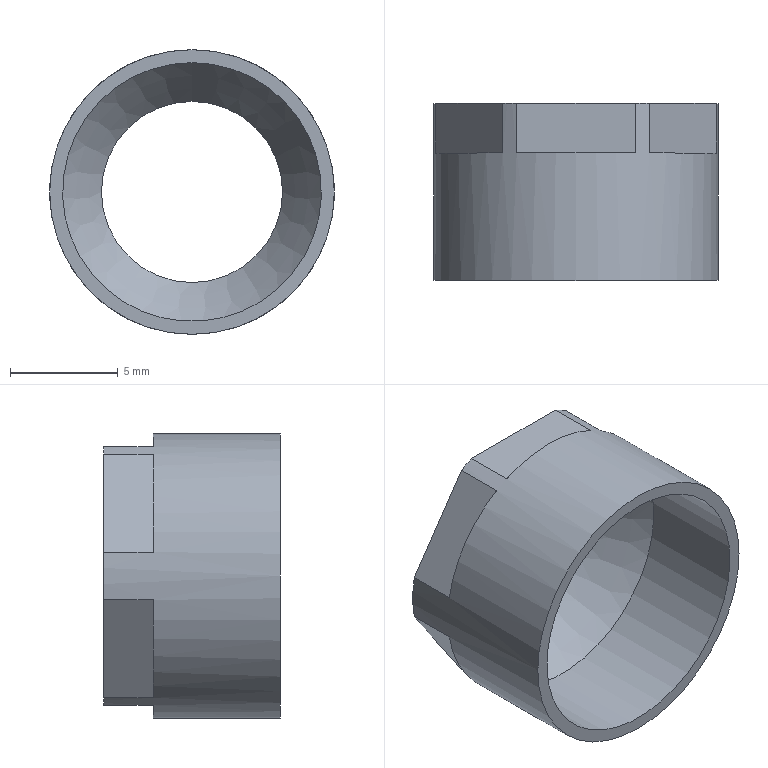Part | STEP file | 1 solid | 18 faces | box 13.2 x 8.2 x 13.2 mm | volume 283.542 mm3 | plane 14 | cylinder 3 | cone 1 | commonest cylinder face diameters 8.4 x1 12 x1 13.2 x1
STEP:
#1=CARTESIAN_POINT('',(0.,0.,0.));
#2=DIRECTION('',(0.,0.,1.));
#3=DIRECTION('',(1.,0.,0.));
#4=AXIS2_PLACEMENT_3D('',#1,#2,#3);
#5=CARTESIAN_POINT('',(0.,0.,6.6));
#6=VERTEX_POINT('',#5);
#7=CARTESIAN_POINT('',(0.,0.,0.));
#8=DIRECTION('',(0.,1.,0.));
#9=DIRECTION('',(0.,0.,1.));
#10=AXIS2_PLACEMENT_3D('',#7,#8,#9);
#11=CIRCLE('',#10,6.6);
#12=CARTESIAN_POINT('',(0.,-0.41,0.));
#13=DIRECTION('',(0.,1.,0.));
#14=DIRECTION('',(0.,0.,1.));
#15=AXIS2_PLACEMENT_3D('',#12,#13,#14);
#16=CYLINDRICAL_SURFACE('',#15,6.6);
#17=CARTESIAN_POINT('',(0.,0.41));
#18=DIRECTION('',(1.,0.));
#19=VECTOR('',#18,1.);
#20=LINE('',#17,#19);
#21=(GEOMETRIC_REPRESENTATION_CONTEXT(2)PARAMETRIC_REPRESENTATION_CONTEXT()REPRESENTATION_CONTEXT('',''));
#22=DEFINITIONAL_REPRESENTATION('',(#20),#21);
#23=PCURVE('',#16,#22);
#24=CARTESIAN_POINT('',(0.,0.,0.));
#25=DIRECTION('',(0.,1.,0.));
#26=DIRECTION('',(0.,0.,1.));
#27=AXIS2_PLACEMENT_3D('',#24,#25,#26);
#28=PLANE('',#27);
#29=CARTESIAN_POINT('',(0.,0.));
#30=DIRECTION('',(1.,0.));
#31=AXIS2_PLACEMENT_2D('',#29,#30);
#32=CIRCLE('',#31,6.6);
#33=(GEOMETRIC_REPRESENTATION_CONTEXT(2)PARAMETRIC_REPRESENTATION_CONTEXT()REPRESENTATION_CONTEXT('',''));
#34=DEFINITIONAL_REPRESENTATION('',(#32),#33);
#35=PCURVE('',#28,#34);
#36=SURFACE_CURVE('',#11,(#23,#35),.PCURVE_S1.);
#37=EDGE_CURVE('',#6,#6,#36,.T.);
#38=ORIENTED_EDGE('',*,*,#37,.T.);
#39=CARTESIAN_POINT('',(0.,5.9,6.6));
#40=VERTEX_POINT('',#39);
#41=CARTESIAN_POINT('',(0.,0.,6.6));
#42=CARTESIAN_POINT('',(0.,5.9,6.6));
#43=B_SPLINE_CURVE_WITH_KNOTS('',1,(#41,#42),.UNSPECIFIED.,.F.,.F.,(2,2),(0.41,6.31),.PIECEWISE_BEZIER_KNOTS.);
#44=CARTESIAN_POINT('',(6.283,0.));
#45=DIRECTION('',(0.,1.));
#46=VECTOR('',#45,1.);
#47=LINE('',#44,#46);
#48=(GEOMETRIC_REPRESENTATION_CONTEXT(2)PARAMETRIC_REPRESENTATION_CONTEXT()REPRESENTATION_CONTEXT('',''));
#49=DEFINITIONAL_REPRESENTATION('',(#47),#48);
#50=PCURVE('',#16,#49);
#51=CARTESIAN_POINT('',(0.,0.));
#52=DIRECTION('',(0.,1.));
#53=VECTOR('',#52,1.);
#54=LINE('',#51,#53);
#55=(GEOMETRIC_REPRESENTATION_CONTEXT(2)PARAMETRIC_REPRESENTATION_CONTEXT()REPRESENTATION_CONTEXT('',''));
#56=DEFINITIONAL_REPRESENTATION('',(#54),#55);
#57=PCURVE('',#16,#56);
#58=SEAM_CURVE('',#43,(#50,#57),.PCURVE_S1.);
#59=EDGE_CURVE('',#6,#40,#58,.T.);
#60=ORIENTED_EDGE('',*,*,#59,.T.);
#61=CARTESIAN_POINT('',(-2.75,5.9,6.));
#62=VERTEX_POINT('',#61);
#63=CARTESIAN_POINT('',(0.,5.9,0.));
#64=DIRECTION('',(0.,-1.,0.));
#65=DIRECTION('',(0.,0.,1.));
#66=AXIS2_PLACEMENT_3D('',#63,#64,#65);
#67=CIRCLE('',#66,6.6);
#68=CARTESIAN_POINT('',(12.566,6.31));
#69=DIRECTION('',(-1.,0.));
#70=VECTOR('',#69,1.);
#71=LINE('',#68,#70);
#72=(GEOMETRIC_REPRESENTATION_CONTEXT(2)PARAMETRIC_REPRESENTATION_CONTEXT()REPRESENTATION_CONTEXT('',''));
#73=DEFINITIONAL_REPRESENTATION('',(#71),#72);
#74=PCURVE('',#16,#73);
#75=CARTESIAN_POINT('',(0.,5.9,0.));
#76=DIRECTION('',(0.,1.,0.));
#77=DIRECTION('',(0.,0.,1.));
#78=AXIS2_PLACEMENT_3D('',#75,#76,#77);
#79=PLANE('',#78);
#80=CARTESIAN_POINT('',(6.6,0.));
#81=CARTESIAN_POINT('',(6.6,-11.432));
#82=CARTESIAN_POINT('',(-3.3,-5.716));
#83=CARTESIAN_POINT('',(-13.2,0.));
#84=CARTESIAN_POINT('',(-3.3,5.716));
#85=CARTESIAN_POINT('',(6.6,11.432));
#86=CARTESIAN_POINT('',(6.6,0.));
#87=(BOUNDED_CURVE()B_SPLINE_CURVE(2,(#80,#81,#82,#83,#84,#85,#86),.UNSPECIFIED.,.T.,.F.)B_SPLINE_CURVE_WITH_KNOTS((1,2,2,2,2,1),(-2.094,0.,2.094,4.189,6.283,8.378),.UNSPECIFIED.)CURVE()GEOMETRIC_REPRESENTATION_ITEM()RATIONAL_B_SPLINE_CURVE((1.,0.5,1.,0.5,1.,0.5,1.))REPRESENTATION_ITEM(''));
#88=(GEOMETRIC_REPRESENTATION_CONTEXT(2)PARAMETRIC_REPRESENTATION_CONTEXT()REPRESENTATION_CONTEXT('',''));
#89=DEFINITIONAL_REPRESENTATION('',(#87),#88);
#90=PCURVE('',#79,#89);
#91=SURFACE_CURVE('',#67,(#74,#90),.PCURVE_S1.);
#92=EDGE_CURVE('',#40,#62,#91,.T.);
#93=ORIENTED_EDGE('',*,*,#92,.T.);
#94=CARTESIAN_POINT('',(-2.75,8.2,6.));
#95=VERTEX_POINT('',#94);
#96=CARTESIAN_POINT('',(-2.75,-0.41,6.));
#97=DIRECTION('',(0.,1.,0.));
#98=VECTOR('',#97,1.);
#99=LINE('',#96,#98);
#100=CARTESIAN_POINT('',(5.853,0.));
#101=DIRECTION('',(0.,1.));
#102=VECTOR('',#101,1.);
#103=LINE('',#100,#102);
#104=(GEOMETRIC_REPRESENTATION_CONTEXT(2)PARAMETRIC_REPRESENTATION_CONTEXT()REPRESENTATION_CONTEXT('',''));
#105=DEFINITIONAL_REPRESENTATION('',(#103),#104);
#106=PCURVE('',#16,#105);
#107=CARTESIAN_POINT('',(3.169,8.2,6.));
#108=DIRECTION('',(0.,0.,-1.));
#109=DIRECTION('',(-1.,0.,0.));
#110=AXIS2_PLACEMENT_3D('',#107,#108,#109);
#111=PLANE('',#110);
#112=CARTESIAN_POINT('',(5.919,-8.61));
#113=DIRECTION('',(0.,1.));
#114=VECTOR('',#113,1.);
#115=LINE('',#112,#114);
#116=(GEOMETRIC_REPRESENTATION_CONTEXT(2)PARAMETRIC_REPRESENTATION_CONTEXT()REPRESENTATION_CONTEXT('',''));
#117=DEFINITIONAL_REPRESENTATION('',(#115),#116);
#118=PCURVE('',#111,#117);
#119=SURFACE_CURVE('',#99,(#106,#118),.PCURVE_S1.);
#120=EDGE_CURVE('',#62,#95,#119,.T.);
#121=ORIENTED_EDGE('',*,*,#120,.T.);
#122=CARTESIAN_POINT('',(-3.406,8.2,5.653));
#123=VERTEX_POINT('',#122);
#124=CARTESIAN_POINT('',(0.,8.2,0.));
#125=DIRECTION('',(0.,-1.,0.));
#126=DIRECTION('',(0.,0.,1.));
#127=AXIS2_PLACEMENT_3D('',#124,#125,#126);
#128=CIRCLE('',#127,6.6);
#129=CARTESIAN_POINT('',(6.283,8.61));
#130=DIRECTION('',(-1.,0.));
#131=VECTOR('',#130,1.);
#132=LINE('',#129,#131);
#133=(GEOMETRIC_REPRESENTATION_CONTEXT(2)PARAMETRIC_REPRESENTATION_CONTEXT()REPRESENTATION_CONTEXT('',''));
#134=DEFINITIONAL_REPRESENTATION('',(#132),#133);
#135=PCURVE('',#16,#134);
#136=CARTESIAN_POINT('',(0.,8.2,0.));
#137=DIRECTION('',(0.,1.,0.));
#138=DIRECTION('',(0.,0.,1.));
#139=AXIS2_PLACEMENT_3D('',#136,#137,#138);
#140=PLANE('',#139);
#141=CARTESIAN_POINT('',(6.6,0.));
#142=CARTESIAN_POINT('',(6.6,-11.432));
#143=CARTESIAN_POINT('',(-3.3,-5.716));
#144=CARTESIAN_POINT('',(-13.2,0.));
#145=CARTESIAN_POINT('',(-3.3,5.716));
#146=CARTESIAN_POINT('',(6.6,11.432));
#147=CARTESIAN_POINT('',(6.6,0.));
#148=(BOUNDED_CURVE()B_SPLINE_CURVE(2,(#141,#142,#143,#144,#145,#146,#147),.UNSPECIFIED.,.T.,.F.)B_SPLINE_CURVE_WITH_KNOTS((1,2,2,2,2,1),(-2.094,0.,2.094,4.189,6.283,8.378),.UNSPECIFIED.)CURVE()GEOMETRIC_REPRESENTATION_ITEM()RATIONAL_B_SPLINE_CURVE((1.,0.5,1.,0.5,1.,0.5,1.))REPRESENTATION_ITEM(''));
#149=(GEOMETRIC_REPRESENTATION_CONTEXT(2)PARAMETRIC_REPRESENTATION_CONTEXT()REPRESENTATION_CONTEXT('',''));
#150=DEFINITIONAL_REPRESENTATION('',(#148),#149);
#151=PCURVE('',#140,#150);
#152=SURFACE_CURVE('',#128,(#135,#151),.PCURVE_S1.);
#153=EDGE_CURVE('',#95,#123,#152,.T.);
#154=ORIENTED_EDGE('',*,*,#153,.T.);
#155=CARTESIAN_POINT('',(-3.406,5.9,5.653));
#156=VERTEX_POINT('',#155);
#157=CARTESIAN_POINT('',(-3.406,-0.41,5.653));
#158=DIRECTION('',(0.,-1.,0.));
#159=VECTOR('',#158,1.);
#160=LINE('',#157,#159);
#161=CARTESIAN_POINT('',(5.741,0.));
#162=DIRECTION('',(0.,-1.));
#163=VECTOR('',#162,1.);
#164=LINE('',#161,#163);
#165=(GEOMETRIC_REPRESENTATION_CONTEXT(2)PARAMETRIC_REPRESENTATION_CONTEXT()REPRESENTATION_CONTEXT('',''));
#166=DEFINITIONAL_REPRESENTATION('',(#164),#165);
#167=PCURVE('',#16,#166);
#168=CARTESIAN_POINT('',(-3.169,8.2,6.));
#169=DIRECTION('',(0.826,0.,-0.5637));
#170=DIRECTION('',(-0.5637,0.,-0.826));
#171=AXIS2_PLACEMENT_3D('',#168,#169,#170);
#172=PLANE('',#171);
#173=CARTESIAN_POINT('',(0.4196,-8.61));
#174=DIRECTION('',(0.,-1.));
#175=VECTOR('',#174,1.);
#176=LINE('',#173,#175);
#177=(GEOMETRIC_REPRESENTATION_CONTEXT(2)PARAMETRIC_REPRESENTATION_CONTEXT()REPRESENTATION_CONTEXT('',''));
#178=DEFINITIONAL_REPRESENTATION('',(#176),#177);
#179=PCURVE('',#172,#178);
#180=SURFACE_CURVE('',#160,(#167,#179),.PCURVE_S1.);
#181=EDGE_CURVE('',#123,#156,#180,.T.);
#182=ORIENTED_EDGE('',*,*,#181,.T.);
#183=CARTESIAN_POINT('',(-6.506,5.9,1.111));
#184=VERTEX_POINT('',#183);
#185=CARTESIAN_POINT('',(0.,5.9,0.));
#186=DIRECTION('',(0.,-1.,0.));
#187=DIRECTION('',(0.,0.,1.));
#188=AXIS2_PLACEMENT_3D('',#185,#186,#187);
#189=CIRCLE('',#188,6.6);
#190=CARTESIAN_POINT('',(6.283,6.31));
#191=DIRECTION('',(-1.,0.));
#192=VECTOR('',#191,1.);
#193=LINE('',#190,#192);
#194=(GEOMETRIC_REPRESENTATION_CONTEXT(2)PARAMETRIC_REPRESENTATION_CONTEXT()REPRESENTATION_CONTEXT('',''));
#195=DEFINITIONAL_REPRESENTATION('',(#193),#194);
#196=PCURVE('',#16,#195);
#197=CARTESIAN_POINT('',(0.,5.9,0.));
#198=DIRECTION('',(0.,1.,0.));
#199=DIRECTION('',(0.,0.,1.));
#200=AXIS2_PLACEMENT_3D('',#197,#198,#199);
#201=PLANE('',#200);
#202=CARTESIAN_POINT('',(6.6,0.));
#203=CARTESIAN_POINT('',(6.6,-11.432));
#204=CARTESIAN_POINT('',(-3.3,-5.716));
#205=CARTESIAN_POINT('',(-13.2,0.));
#206=CARTESIAN_POINT('',(-3.3,5.716));
#207=CARTESIAN_POINT('',(6.6,11.432));
#208=CARTESIAN_POINT('',(6.6,0.));
#209=(BOUNDED_CURVE()B_SPLINE_CURVE(2,(#202,#203,#204,#205,#206,#207,#208),.UNSPECIFIED.,.T.,.F.)B_SPLINE_CURVE_WITH_KNOTS((1,2,2,2,2,1),(-2.094,0.,2.094,4.189,6.283,8.378),.UNSPECIFIED.)CURVE()GEOMETRIC_REPRESENTATION_ITEM()RATIONAL_B_SPLINE_CURVE((1.,0.5,1.,0.5,1.,0.5,1.))REPRESENTATION_ITEM(''));
#210=(GEOMETRIC_REPRESENTATION_CONTEXT(2)PARAMETRIC_REPRESENTATION_CONTEXT()REPRESENTATION_CONTEXT('',''));
#211=DEFINITIONAL_REPRESENTATION('',(#209),#210);
#212=PCURVE('',#201,#211);
#213=SURFACE_CURVE('',#189,(#196,#212),.PCURVE_S1.);
#214=EDGE_CURVE('',#156,#184,#213,.T.);
#215=ORIENTED_EDGE('',*,*,#214,.T.);
#216=CARTESIAN_POINT('',(-6.506,8.2,1.111));
#217=VERTEX_POINT('',#216);
#218=CARTESIAN_POINT('',(-6.506,-0.41,1.111));
#219=DIRECTION('',(0.,1.,0.));
#220=VECTOR('',#219,1.);
#221=LINE('',#218,#220);
#222=CARTESIAN_POINT('',(4.882,0.));
#223=DIRECTION('',(0.,1.));
#224=VECTOR('',#223,1.);
#225=LINE('',#222,#224);
#226=(GEOMETRIC_REPRESENTATION_CONTEXT(2)PARAMETRIC_REPRESENTATION_CONTEXT()REPRESENTATION_CONTEXT('',''));
#227=DEFINITIONAL_REPRESENTATION('',(#225),#226);
#228=PCURVE('',#16,#227);
#229=CARTESIAN_POINT('',(5.919,-8.61));
#230=DIRECTION('',(0.,1.));
#231=VECTOR('',#230,1.);
#232=LINE('',#229,#231);
#233=(GEOMETRIC_REPRESENTATION_CONTEXT(2)PARAMETRIC_REPRESENTATION_CONTEXT()REPRESENTATION_CONTEXT('',''));
#234=DEFINITIONAL_REPRESENTATION('',(#232),#233);
#235=PCURVE('',#172,#234);
#236=SURFACE_CURVE('',#221,(#228,#235),.PCURVE_S1.);
#237=EDGE_CURVE('',#184,#217,#236,.T.);
#238=ORIENTED_EDGE('',*,*,#237,.T.);
#239=CARTESIAN_POINT('',(-6.506,8.2,-1.111));
#240=VERTEX_POINT('',#239);
#241=CARTESIAN_POINT('',(0.,8.2,0.));
#242=DIRECTION('',(0.,-1.,0.));
#243=DIRECTION('',(0.,0.,1.));
#244=AXIS2_PLACEMENT_3D('',#241,#242,#243);
#245=CIRCLE('',#244,6.6);
#246=CARTESIAN_POINT('',(6.283,8.61));
#247=DIRECTION('',(-1.,0.));
#248=VECTOR('',#247,1.);
#249=LINE('',#246,#248);
#250=(GEOMETRIC_REPRESENTATION_CONTEXT(2)PARAMETRIC_REPRESENTATION_CONTEXT()REPRESENTATION_CONTEXT('',''));
#251=DEFINITIONAL_REPRESENTATION('',(#249),#250);
#252=PCURVE('',#16,#251);
#253=CARTESIAN_POINT('',(6.6,0.));
#254=CARTESIAN_POINT('',(6.6,-11.432));
#255=CARTESIAN_POINT('',(-3.3,-5.716));
#256=CARTESIAN_POINT('',(-13.2,0.));
#257=CARTESIAN_POINT('',(-3.3,5.716));
#258=CARTESIAN_POINT('',(6.6,11.432));
#259=CARTESIAN_POINT('',(6.6,0.));
#260=(BOUNDED_CURVE()B_SPLINE_CURVE(2,(#253,#254,#255,#256,#257,#258,#259),.UNSPECIFIED.,.T.,.F.)B_SPLINE_CURVE_WITH_KNOTS((1,2,2,2,2,1),(-2.094,0.,2.094,4.189,6.283,8.378),.UNSPECIFIED.)CURVE()GEOMETRIC_REPRESENTATION_ITEM()RATIONAL_B_SPLINE_CURVE((1.,0.5,1.,0.5,1.,0.5,1.))REPRESENTATION_ITEM(''));
#261=(GEOMETRIC_REPRESENTATION_CONTEXT(2)PARAMETRIC_REPRESENTATION_CONTEXT()REPRESENTATION_CONTEXT('',''));
#262=DEFINITIONAL_REPRESENTATION('',(#260),#261);
#263=PCURVE('',#140,#262);
#264=SURFACE_CURVE('',#245,(#252,#263),.PCURVE_S1.);
#265=EDGE_CURVE('',#217,#240,#264,.T.);
#266=ORIENTED_EDGE('',*,*,#265,.T.);
#267=CARTESIAN_POINT('',(-6.506,5.9,-1.111));
#268=VERTEX_POINT('',#267);
#269=CARTESIAN_POINT('',(-6.506,-0.41,-1.111));
#270=DIRECTION('',(0.,-1.,0.));
#271=VECTOR('',#270,1.);
#272=LINE('',#269,#271);
#273=CARTESIAN_POINT('',(4.543,0.));
#274=DIRECTION('',(0.,-1.));
#275=VECTOR('',#274,1.);
#276=LINE('',#273,#275);
#277=(GEOMETRIC_REPRESENTATION_CONTEXT(2)PARAMETRIC_REPRESENTATION_CONTEXT()REPRESENTATION_CONTEXT('',''));
#278=DEFINITIONAL_REPRESENTATION('',(#276),#277);
#279=PCURVE('',#16,#278);
#280=CARTESIAN_POINT('',(-7.264,8.2,0.));
#281=DIRECTION('',(0.826,0.,0.5637));
#282=DIRECTION('',(0.5637,0.,-0.826));
#283=AXIS2_PLACEMENT_3D('',#280,#281,#282);
#284=PLANE('',#283);
#285=CARTESIAN_POINT('',(1.346,-8.61));
#286=DIRECTION('',(0.,-1.));
#287=VECTOR('',#286,1.);
#288=LINE('',#285,#287);
#289=(GEOMETRIC_REPRESENTATION_CONTEXT(2)PARAMETRIC_REPRESENTATION_CONTEXT()REPRESENTATION_CONTEXT('',''));
#290=DEFINITIONAL_REPRESENTATION('',(#288),#289);
#291=PCURVE('',#284,#290);
#292=SURFACE_CURVE('',#272,(#279,#291),.PCURVE_S1.);
#293=EDGE_CURVE('',#240,#268,#292,.T.);
#294=ORIENTED_EDGE('',*,*,#293,.T.);
#295=CARTESIAN_POINT('',(-3.406,5.9,-5.653));
#296=VERTEX_POINT('',#295);
#297=CARTESIAN_POINT('',(0.,5.9,0.));
#298=DIRECTION('',(0.,-1.,0.));
#299=DIRECTION('',(0.,0.,1.));
#300=AXIS2_PLACEMENT_3D('',#297,#298,#299);
#301=CIRCLE('',#300,6.6);
#302=CARTESIAN_POINT('',(6.283,6.31));
#303=DIRECTION('',(-1.,0.));
#304=VECTOR('',#303,1.);
#305=LINE('',#302,#304);
#306=(GEOMETRIC_REPRESENTATION_CONTEXT(2)PARAMETRIC_REPRESENTATION_CONTEXT()REPRESENTATION_CONTEXT('',''));
#307=DEFINITIONAL_REPRESENTATION('',(#305),#306);
#308=PCURVE('',#16,#307);
#309=CARTESIAN_POINT('',(0.,5.9,0.));
#310=DIRECTION('',(0.,1.,0.));
#311=DIRECTION('',(0.,0.,1.));
#312=AXIS2_PLACEMENT_3D('',#309,#310,#311);
#313=PLANE('',#312);
#314=CARTESIAN_POINT('',(6.6,0.));
#315=CARTESIAN_POINT('',(6.6,-11.432));
#316=CARTESIAN_POINT('',(-3.3,-5.716));
#317=CARTESIAN_POINT('',(-13.2,0.));
#318=CARTESIAN_POINT('',(-3.3,5.716));
#319=CARTESIAN_POINT('',(6.6,11.432));
#320=CARTESIAN_POINT('',(6.6,0.));
#321=(BOUNDED_CURVE()B_SPLINE_CURVE(2,(#314,#315,#316,#317,#318,#319,#320),.UNSPECIFIED.,.T.,.F.)B_SPLINE_CURVE_WITH_KNOTS((1,2,2,2,2,1),(-2.094,0.,2.094,4.189,6.283,8.378),.UNSPECIFIED.)CURVE()GEOMETRIC_REPRESENTATION_ITEM()RATIONAL_B_SPLINE_CURVE((1.,0.5,1.,0.5,1.,0.5,1.))REPRESENTATION_ITEM(''));
#322=(GEOMETRIC_REPRESENTATION_CONTEXT(2)PARAMETRIC_REPRESENTATION_CONTEXT()REPRESENTATION_CONTEXT('',''));
#323=DEFINITIONAL_REPRESENTATION('',(#321),#322);
#324=PCURVE('',#313,#323);
#325=SURFACE_CURVE('',#301,(#308,#324),.PCURVE_S1.);
#326=EDGE_CURVE('',#268,#296,#325,.T.);
#327=ORIENTED_EDGE('',*,*,#326,.T.);
#328=CARTESIAN_POINT('',(-3.406,8.2,-5.653));
#329=VERTEX_POINT('',#328);
#330=CARTESIAN_POINT('',(-3.406,-0.41,-5.653));
#331=DIRECTION('',(0.,1.,0.));
#332=VECTOR('',#331,1.);
#333=LINE('',#330,#332);
#334=CARTESIAN_POINT('',(3.684,0.));
#335=DIRECTION('',(0.,1.));
#336=VECTOR('',#335,1.);
#337=LINE('',#334,#336);
#338=(GEOMETRIC_REPRESENTATION_CONTEXT(2)PARAMETRIC_REPRESENTATION_CONTEXT()REPRESENTATION_CONTEXT('',''));
#339=DEFINITIONAL_REPRESENTATION('',(#337),#338);
#340=PCURVE('',#16,#339);
#341=CARTESIAN_POINT('',(6.845,-8.61));
#342=DIRECTION('',(0.,1.));
#343=VECTOR('',#342,1.);
#344=LINE('',#341,#343);
#345=(GEOMETRIC_REPRESENTATION_CONTEXT(2)PARAMETRIC_REPRESENTATION_CONTEXT()REPRESENTATION_CONTEXT('',''));
#346=DEFINITIONAL_REPRESENTATION('',(#344),#345);
#347=PCURVE('',#284,#346);
#348=SURFACE_CURVE('',#333,(#340,#347),.PCURVE_S1.);
#349=EDGE_CURVE('',#296,#329,#348,.T.);
#350=ORIENTED_EDGE('',*,*,#349,.T.);
#351=CARTESIAN_POINT('',(-2.75,8.2,-6.));
#352=VERTEX_POINT('',#351);
#353=CARTESIAN_POINT('',(0.,8.2,0.));
#354=DIRECTION('',(0.,1.,0.));
#355=DIRECTION('',(0.,0.,1.));
#356=AXIS2_PLACEMENT_3D('',#353,#354,#355);
#357=CIRCLE('',#356,6.6);
#358=CARTESIAN_POINT('',(0.,8.61));
#359=DIRECTION('',(1.,0.));
#360=VECTOR('',#359,1.);
#361=LINE('',#358,#360);
#362=(GEOMETRIC_REPRESENTATION_CONTEXT(2)PARAMETRIC_REPRESENTATION_CONTEXT()REPRESENTATION_CONTEXT('',''));
#363=DEFINITIONAL_REPRESENTATION('',(#361),#362);
#364=PCURVE('',#16,#363);
#365=CARTESIAN_POINT('',(0.,0.));
#366=DIRECTION('',(1.,0.));
#367=AXIS2_PLACEMENT_2D('',#365,#366);
#368=CIRCLE('',#367,6.6);
#369=(GEOMETRIC_REPRESENTATION_CONTEXT(2)PARAMETRIC_REPRESENTATION_CONTEXT()REPRESENTATION_CONTEXT('',''));
#370=DEFINITIONAL_REPRESENTATION('',(#368),#369);
#371=PCURVE('',#140,#370);
#372=SURFACE_CURVE('',#357,(#364,#371),.PCURVE_S1.);
#373=EDGE_CURVE('',#352,#329,#372,.T.);
#374=ORIENTED_EDGE('',*,*,#373,.F.);
#375=CARTESIAN_POINT('',(-2.75,5.9,-6.));
#376=VERTEX_POINT('',#375);
#377=CARTESIAN_POINT('',(-2.75,-0.41,-6.));
#378=DIRECTION('',(0.,-1.,0.));
#379=VECTOR('',#378,1.);
#380=LINE('',#377,#379);
#381=CARTESIAN_POINT('',(3.571,0.));
#382=DIRECTION('',(0.,-1.));
#383=VECTOR('',#382,1.);
#384=LINE('',#381,#383);
#385=(GEOMETRIC_REPRESENTATION_CONTEXT(2)PARAMETRIC_REPRESENTATION_CONTEXT()REPRESENTATION_CONTEXT('',''));
#386=DEFINITIONAL_REPRESENTATION('',(#384),#385);
#387=PCURVE('',#16,#386);
#388=CARTESIAN_POINT('',(-3.169,8.2,-6.));
#389=DIRECTION('',(0.,0.,1.));
#390=DIRECTION('',(1.,0.,0.));
#391=AXIS2_PLACEMENT_3D('',#388,#389,#390);
#392=PLANE('',#391);
#393=CARTESIAN_POINT('',(0.4196,-8.61));
#394=DIRECTION('',(0.,-1.));
#395=VECTOR('',#394,1.);
#396=LINE('',#393,#395);
#397=(GEOMETRIC_REPRESENTATION_CONTEXT(2)PARAMETRIC_REPRESENTATION_CONTEXT()REPRESENTATION_CONTEXT('',''));
#398=DEFINITIONAL_REPRESENTATION('',(#396),#397);
#399=PCURVE('',#392,#398);
#400=SURFACE_CURVE('',#380,(#387,#399),.PCURVE_S1.);
#401=EDGE_CURVE('',#352,#376,#400,.T.);
#402=ORIENTED_EDGE('',*,*,#401,.T.);
#403=CARTESIAN_POINT('',(2.75,5.9,-6.));
#404=VERTEX_POINT('',#403);
#405=CARTESIAN_POINT('',(0.,5.9,0.));
#406=DIRECTION('',(0.,-1.,0.));
#407=DIRECTION('',(0.,0.,1.));
#408=AXIS2_PLACEMENT_3D('',#405,#406,#407);
#409=CIRCLE('',#408,6.6);
#410=CARTESIAN_POINT('',(6.283,6.31));
#411=DIRECTION('',(-1.,0.));
#412=VECTOR('',#411,1.);
#413=LINE('',#410,#412);
#414=(GEOMETRIC_REPRESENTATION_CONTEXT(2)PARAMETRIC_REPRESENTATION_CONTEXT()REPRESENTATION_CONTEXT('',''));
#415=DEFINITIONAL_REPRESENTATION('',(#413),#414);
#416=PCURVE('',#16,#415);
#417=CARTESIAN_POINT('',(0.,5.9,0.));
#418=DIRECTION('',(0.,1.,0.));
#419=DIRECTION('',(0.,0.,1.));
#420=AXIS2_PLACEMENT_3D('',#417,#418,#419);
#421=PLANE('',#420);
#422=CARTESIAN_POINT('',(6.6,0.));
#423=CARTESIAN_POINT('',(6.6,-11.432));
#424=CARTESIAN_POINT('',(-3.3,-5.716));
#425=CARTESIAN_POINT('',(-13.2,0.));
#426=CARTESIAN_POINT('',(-3.3,5.716));
#427=CARTESIAN_POINT('',(6.6,11.432));
#428=CARTESIAN_POINT('',(6.6,0.));
#429=(BOUNDED_CURVE()B_SPLINE_CURVE(2,(#422,#423,#424,#425,#426,#427,#428),.UNSPECIFIED.,.T.,.F.)B_SPLINE_CURVE_WITH_KNOTS((1,2,2,2,2,1),(-2.094,0.,2.094,4.189,6.283,8.378),.UNSPECIFIED.)CURVE()GEOMETRIC_REPRESENTATION_ITEM()RATIONAL_B_SPLINE_CURVE((1.,0.5,1.,0.5,1.,0.5,1.))REPRESENTATION_ITEM(''));
#430=(GEOMETRIC_REPRESENTATION_CONTEXT(2)PARAMETRIC_REPRESENTATION_CONTEXT()REPRESENTATION_CONTEXT('',''));
#431=DEFINITIONAL_REPRESENTATION('',(#429),#430);
#432=PCURVE('',#421,#431);
#433=SURFACE_CURVE('',#409,(#416,#432),.PCURVE_S1.);
#434=EDGE_CURVE('',#376,#404,#433,.T.);
#435=ORIENTED_EDGE('',*,*,#434,.T.);
#436=CARTESIAN_POINT('',(2.75,8.2,-6.));
#437=VERTEX_POINT('',#436);
#438=CARTESIAN_POINT('',(2.75,8.2,-6.));
#439=DIRECTION('',(0.,1.,0.));
#440=VECTOR('',#439,1.);
#441=LINE('',#438,#440);
#442=CARTESIAN_POINT('',(2.712,8.61));
#443=DIRECTION('',(0.,1.));
#444=VECTOR('',#443,1.);
#445=LINE('',#442,#444);
#446=(GEOMETRIC_REPRESENTATION_CONTEXT(2)PARAMETRIC_REPRESENTATION_CONTEXT()REPRESENTATION_CONTEXT('',''));
#447=DEFINITIONAL_REPRESENTATION('',(#445),#446);
#448=PCURVE('',#16,#447);
#449=CARTESIAN_POINT('',(5.919,0.));
#450=DIRECTION('',(0.,1.));
#451=VECTOR('',#450,1.);
#452=LINE('',#449,#451);
#453=(GEOMETRIC_REPRESENTATION_CONTEXT(2)PARAMETRIC_REPRESENTATION_CONTEXT()REPRESENTATION_CONTEXT('',''));
#454=DEFINITIONAL_REPRESENTATION('',(#452),#453);
#455=PCURVE('',#392,#454);
#456=SURFACE_CURVE('',#441,(#448,#455),.PCURVE_S1.);
#457=EDGE_CURVE('',#404,#437,#456,.T.);
#458=ORIENTED_EDGE('',*,*,#457,.T.);
#459=CARTESIAN_POINT('',(3.406,8.2,-5.653));
#460=VERTEX_POINT('',#459);
#461=CARTESIAN_POINT('',(0.,8.2,0.));
#462=DIRECTION('',(0.,1.,0.));
#463=DIRECTION('',(0.,0.,1.));
#464=AXIS2_PLACEMENT_3D('',#461,#462,#463);
#465=CIRCLE('',#464,6.6);
#466=CARTESIAN_POINT('',(0.,8.61));
#467=DIRECTION('',(1.,0.));
#468=VECTOR('',#467,1.);
#469=LINE('',#466,#468);
#470=(GEOMETRIC_REPRESENTATION_CONTEXT(2)PARAMETRIC_REPRESENTATION_CONTEXT()REPRESENTATION_CONTEXT('',''));
#471=DEFINITIONAL_REPRESENTATION('',(#469),#470);
#472=PCURVE('',#16,#471);
#473=CARTESIAN_POINT('',(0.,0.));
#474=DIRECTION('',(1.,0.));
#475=AXIS2_PLACEMENT_2D('',#473,#474);
#476=CIRCLE('',#475,6.6);
#477=(GEOMETRIC_REPRESENTATION_CONTEXT(2)PARAMETRIC_REPRESENTATION_CONTEXT()REPRESENTATION_CONTEXT('',''));
#478=DEFINITIONAL_REPRESENTATION('',(#476),#477);
#479=PCURVE('',#140,#478);
#480=SURFACE_CURVE('',#465,(#472,#479),.PCURVE_S1.);
#481=EDGE_CURVE('',#460,#437,#480,.T.);
#482=ORIENTED_EDGE('',*,*,#481,.F.);
#483=CARTESIAN_POINT('',(3.406,5.9,-5.653));
#484=VERTEX_POINT('',#483);
#485=CARTESIAN_POINT('',(3.406,-0.41,-5.653));
#486=DIRECTION('',(0.,-1.,0.));
#487=VECTOR('',#486,1.);
#488=LINE('',#485,#487);
#489=CARTESIAN_POINT('',(2.599,0.));
#490=DIRECTION('',(0.,-1.));
#491=VECTOR('',#490,1.);
#492=LINE('',#489,#491);
#493=(GEOMETRIC_REPRESENTATION_CONTEXT(2)PARAMETRIC_REPRESENTATION_CONTEXT()REPRESENTATION_CONTEXT('',''));
#494=DEFINITIONAL_REPRESENTATION('',(#492),#493);
#495=PCURVE('',#16,#494);
#496=CARTESIAN_POINT('',(3.169,8.2,-6.));
#497=DIRECTION('',(-0.826,0.,0.5637));
#498=DIRECTION('',(0.5637,0.,0.826));
#499=AXIS2_PLACEMENT_3D('',#496,#497,#498);
#500=PLANE('',#499);
#501=CARTESIAN_POINT('',(0.4196,-8.61));
#502=DIRECTION('',(0.,-1.));
#503=VECTOR('',#502,1.);
#504=LINE('',#501,#503);
#505=(GEOMETRIC_REPRESENTATION_CONTEXT(2)PARAMETRIC_REPRESENTATION_CONTEXT()REPRESENTATION_CONTEXT('',''));
#506=DEFINITIONAL_REPRESENTATION('',(#504),#505);
#507=PCURVE('',#500,#506);
#508=SURFACE_CURVE('',#488,(#495,#507),.PCURVE_S1.);
#509=EDGE_CURVE('',#460,#484,#508,.T.);
#510=ORIENTED_EDGE('',*,*,#509,.T.);
#511=CARTESIAN_POINT('',(6.506,5.9,-1.111));
#512=VERTEX_POINT('',#511);
#513=CARTESIAN_POINT('',(0.,5.9,0.));
#514=DIRECTION('',(0.,-1.,0.));
#515=DIRECTION('',(0.,0.,1.));
#516=AXIS2_PLACEMENT_3D('',#513,#514,#515);
#517=CIRCLE('',#516,6.6);
#518=CARTESIAN_POINT('',(6.283,6.31));
#519=DIRECTION('',(-1.,0.));
#520=VECTOR('',#519,1.);
#521=LINE('',#518,#520);
#522=(GEOMETRIC_REPRESENTATION_CONTEXT(2)PARAMETRIC_REPRESENTATION_CONTEXT()REPRESENTATION_CONTEXT('',''));
#523=DEFINITIONAL_REPRESENTATION('',(#521),#522);
#524=PCURVE('',#16,#523);
#525=CARTESIAN_POINT('',(0.,5.9,0.));
#526=DIRECTION('',(0.,1.,0.));
#527=DIRECTION('',(0.,0.,1.));
#528=AXIS2_PLACEMENT_3D('',#525,#526,#527);
#529=PLANE('',#528);
#530=CARTESIAN_POINT('',(6.6,0.));
#531=CARTESIAN_POINT('',(6.6,-11.432));
#532=CARTESIAN_POINT('',(-3.3,-5.716));
#533=CARTESIAN_POINT('',(-13.2,0.));
#534=CARTESIAN_POINT('',(-3.3,5.716));
#535=CARTESIAN_POINT('',(6.6,11.432));
#536=CARTESIAN_POINT('',(6.6,0.));
#537=(BOUNDED_CURVE()B_SPLINE_CURVE(2,(#530,#531,#532,#533,#534,#535,#536),.UNSPECIFIED.,.T.,.F.)B_SPLINE_CURVE_WITH_KNOTS((1,2,2,2,2,1),(-2.094,0.,2.094,4.189,6.283,8.378),.UNSPECIFIED.)CURVE()GEOMETRIC_REPRESENTATION_ITEM()RATIONAL_B_SPLINE_CURVE((1.,0.5,1.,0.5,1.,0.5,1.))REPRESENTATION_ITEM(''));
#538=(GEOMETRIC_REPRESENTATION_CONTEXT(2)PARAMETRIC_REPRESENTATION_CONTEXT()REPRESENTATION_CONTEXT('',''));
#539=DEFINITIONAL_REPRESENTATION('',(#537),#538);
#540=PCURVE('',#529,#539);
#541=SURFACE_CURVE('',#517,(#524,#540),.PCURVE_S1.);
#542=EDGE_CURVE('',#484,#512,#541,.T.);
#543=ORIENTED_EDGE('',*,*,#542,.T.);
#544=CARTESIAN_POINT('',(6.506,8.2,-1.111));
#545=VERTEX_POINT('',#544);
#546=CARTESIAN_POINT('',(6.506,-0.41,-1.111));
#547=DIRECTION('',(0.,1.,0.));
#548=VECTOR('',#547,1.);
#549=LINE('',#546,#548);
#550=CARTESIAN_POINT('',(1.74,0.));
#551=DIRECTION('',(0.,1.));
#552=VECTOR('',#551,1.);
#553=LINE('',#550,#552);
#554=(GEOMETRIC_REPRESENTATION_CONTEXT(2)PARAMETRIC_REPRESENTATION_CONTEXT()REPRESENTATION_CONTEXT('',''));
#555=DEFINITIONAL_REPRESENTATION('',(#553),#554);
#556=PCURVE('',#16,#555);
#557=CARTESIAN_POINT('',(5.919,-8.61));
#558=DIRECTION('',(0.,1.));
#559=VECTOR('',#558,1.);
#560=LINE('',#557,#559);
#561=(GEOMETRIC_REPRESENTATION_CONTEXT(2)PARAMETRIC_REPRESENTATION_CONTEXT()REPRESENTATION_CONTEXT('',''));
#562=DEFINITIONAL_REPRESENTATION('',(#560),#561);
#563=PCURVE('',#500,#562);
#564=SURFACE_CURVE('',#549,(#556,#563),.PCURVE_S1.);
#565=EDGE_CURVE('',#512,#545,#564,.T.);
#566=ORIENTED_EDGE('',*,*,#565,.T.);
#567=CARTESIAN_POINT('',(6.506,8.2,1.111));
#568=VERTEX_POINT('',#567);
#569=CARTESIAN_POINT('',(0.,8.2,0.));
#570=DIRECTION('',(0.,1.,0.));
#571=DIRECTION('',(0.,0.,1.));
#572=AXIS2_PLACEMENT_3D('',#569,#570,#571);
#573=CIRCLE('',#572,6.6);
#574=CARTESIAN_POINT('',(0.,8.61));
#575=DIRECTION('',(1.,0.));
#576=VECTOR('',#575,1.);
#577=LINE('',#574,#576);
#578=(GEOMETRIC_REPRESENTATION_CONTEXT(2)PARAMETRIC_REPRESENTATION_CONTEXT()REPRESENTATION_CONTEXT('',''));
#579=DEFINITIONAL_REPRESENTATION('',(#577),#578);
#580=PCURVE('',#16,#579);
#581=CARTESIAN_POINT('',(0.,0.));
#582=DIRECTION('',(1.,0.));
#583=AXIS2_PLACEMENT_2D('',#581,#582);
#584=CIRCLE('',#583,6.6);
#585=(GEOMETRIC_REPRESENTATION_CONTEXT(2)PARAMETRIC_REPRESENTATION_CONTEXT()REPRESENTATION_CONTEXT('',''));
#586=DEFINITIONAL_REPRESENTATION('',(#584),#585);
#587=PCURVE('',#140,#586);
#588=SURFACE_CURVE('',#573,(#580,#587),.PCURVE_S1.);
#589=EDGE_CURVE('',#568,#545,#588,.T.);
#590=ORIENTED_EDGE('',*,*,#589,.F.);
#591=CARTESIAN_POINT('',(6.506,5.9,1.111));
#592=VERTEX_POINT('',#591);
#593=CARTESIAN_POINT('',(6.506,-0.41,1.111));
#594=DIRECTION('',(0.,-1.,0.));
#595=VECTOR('',#594,1.);
#596=LINE('',#593,#595);
#597=CARTESIAN_POINT('',(1.402,0.));
#598=DIRECTION('',(0.,-1.));
#599=VECTOR('',#598,1.);
#600=LINE('',#597,#599);
#601=(GEOMETRIC_REPRESENTATION_CONTEXT(2)PARAMETRIC_REPRESENTATION_CONTEXT()REPRESENTATION_CONTEXT('',''));
#602=DEFINITIONAL_REPRESENTATION('',(#600),#601);
#603=PCURVE('',#16,#602);
#604=CARTESIAN_POINT('',(7.264,8.2,0.));
#605=DIRECTION('',(-0.826,0.,-0.5637));
#606=DIRECTION('',(-0.5637,0.,0.826));
#607=AXIS2_PLACEMENT_3D('',#604,#605,#606);
#608=PLANE('',#607);
#609=CARTESIAN_POINT('',(1.346,-8.61));
#610=DIRECTION('',(0.,-1.));
#611=VECTOR('',#610,1.);
#612=LINE('',#609,#611);
#613=(GEOMETRIC_REPRESENTATION_CONTEXT(2)PARAMETRIC_REPRESENTATION_CONTEXT()REPRESENTATION_CONTEXT('',''));
#614=DEFINITIONAL_REPRESENTATION('',(#612),#613);
#615=PCURVE('',#608,#614);
#616=SURFACE_CURVE('',#596,(#603,#615),.PCURVE_S1.);
#617=EDGE_CURVE('',#568,#592,#616,.T.);
#618=ORIENTED_EDGE('',*,*,#617,.T.);
#619=CARTESIAN_POINT('',(3.406,5.9,5.653));
#620=VERTEX_POINT('',#619);
#621=CARTESIAN_POINT('',(0.,5.9,0.));
#622=DIRECTION('',(0.,-1.,0.));
#623=DIRECTION('',(0.,0.,1.));
#624=AXIS2_PLACEMENT_3D('',#621,#622,#623);
#625=CIRCLE('',#624,6.6);
#626=CARTESIAN_POINT('',(6.283,6.31));
#627=DIRECTION('',(-1.,0.));
#628=VECTOR('',#627,1.);
#629=LINE('',#626,#628);
#630=(GEOMETRIC_REPRESENTATION_CONTEXT(2)PARAMETRIC_REPRESENTATION_CONTEXT()REPRESENTATION_CONTEXT('',''));
#631=DEFINITIONAL_REPRESENTATION('',(#629),#630);
#632=PCURVE('',#16,#631);
#633=CARTESIAN_POINT('',(0.,5.9,0.));
#634=DIRECTION('',(0.,1.,0.));
#635=DIRECTION('',(0.,0.,1.));
#636=AXIS2_PLACEMENT_3D('',#633,#634,#635);
#637=PLANE('',#636);
#638=CARTESIAN_POINT('',(6.6,0.));
#639=CARTESIAN_POINT('',(6.6,-11.432));
#640=CARTESIAN_POINT('',(-3.3,-5.716));
#641=CARTESIAN_POINT('',(-13.2,0.));
#642=CARTESIAN_POINT('',(-3.3,5.716));
#643=CARTESIAN_POINT('',(6.6,11.432));
#644=CARTESIAN_POINT('',(6.6,0.));
#645=(BOUNDED_CURVE()B_SPLINE_CURVE(2,(#638,#639,#640,#641,#642,#643,#644),.UNSPECIFIED.,.T.,.F.)B_SPLINE_CURVE_WITH_KNOTS((1,2,2,2,2,1),(-2.094,0.,2.094,4.189,6.283,8.378),.UNSPECIFIED.)CURVE()GEOMETRIC_REPRESENTATION_ITEM()RATIONAL_B_SPLINE_CURVE((1.,0.5,1.,0.5,1.,0.5,1.))REPRESENTATION_ITEM(''));
#646=(GEOMETRIC_REPRESENTATION_CONTEXT(2)PARAMETRIC_REPRESENTATION_CONTEXT()REPRESENTATION_CONTEXT('',''));
#647=DEFINITIONAL_REPRESENTATION('',(#645),#646);
#648=PCURVE('',#637,#647);
#649=SURFACE_CURVE('',#625,(#632,#648),.PCURVE_S1.);
#650=EDGE_CURVE('',#592,#620,#649,.T.);
#651=ORIENTED_EDGE('',*,*,#650,.T.);
#652=CARTESIAN_POINT('',(3.406,8.2,5.653));
#653=VERTEX_POINT('',#652);
#654=CARTESIAN_POINT('',(3.406,-0.41,5.653));
#655=DIRECTION('',(0.,1.,0.));
#656=VECTOR('',#655,1.);
#657=LINE('',#654,#656);
#658=CARTESIAN_POINT('',(0.5422,0.));
#659=DIRECTION('',(0.,1.));
#660=VECTOR('',#659,1.);
#661=LINE('',#658,#660);
#662=(GEOMETRIC_REPRESENTATION_CONTEXT(2)PARAMETRIC_REPRESENTATION_CONTEXT()REPRESENTATION_CONTEXT('',''));
#663=DEFINITIONAL_REPRESENTATION('',(#661),#662);
#664=PCURVE('',#16,#663);
#665=CARTESIAN_POINT('',(6.845,-8.61));
#666=DIRECTION('',(0.,1.));
#667=VECTOR('',#666,1.);
#668=LINE('',#665,#667);
#669=(GEOMETRIC_REPRESENTATION_CONTEXT(2)PARAMETRIC_REPRESENTATION_CONTEXT()REPRESENTATION_CONTEXT('',''));
#670=DEFINITIONAL_REPRESENTATION('',(#668),#669);
#671=PCURVE('',#608,#670);
#672=SURFACE_CURVE('',#657,(#664,#671),.PCURVE_S1.);
#673=EDGE_CURVE('',#620,#653,#672,.T.);
#674=ORIENTED_EDGE('',*,*,#673,.T.);
#675=CARTESIAN_POINT('',(2.75,8.2,6.));
#676=VERTEX_POINT('',#675);
#677=CARTESIAN_POINT('',(0.,8.2,0.));
#678=DIRECTION('',(0.,1.,0.));
#679=DIRECTION('',(0.,0.,1.));
#680=AXIS2_PLACEMENT_3D('',#677,#678,#679);
#681=CIRCLE('',#680,6.6);
#682=CARTESIAN_POINT('',(0.,8.61));
#683=DIRECTION('',(1.,0.));
#684=VECTOR('',#683,1.);
#685=LINE('',#682,#684);
#686=(GEOMETRIC_REPRESENTATION_CONTEXT(2)PARAMETRIC_REPRESENTATION_CONTEXT()REPRESENTATION_CONTEXT('',''));
#687=DEFINITIONAL_REPRESENTATION('',(#685),#686);
#688=PCURVE('',#16,#687);
#689=CARTESIAN_POINT('',(0.,0.));
#690=DIRECTION('',(1.,0.));
#691=AXIS2_PLACEMENT_2D('',#689,#690);
#692=CIRCLE('',#691,6.6);
#693=(GEOMETRIC_REPRESENTATION_CONTEXT(2)PARAMETRIC_REPRESENTATION_CONTEXT()REPRESENTATION_CONTEXT('',''));
#694=DEFINITIONAL_REPRESENTATION('',(#692),#693);
#695=PCURVE('',#140,#694);
#696=SURFACE_CURVE('',#681,(#688,#695),.PCURVE_S1.);
#697=EDGE_CURVE('',#676,#653,#696,.T.);
#698=ORIENTED_EDGE('',*,*,#697,.F.);
#699=CARTESIAN_POINT('',(2.75,5.9,6.));
#700=VERTEX_POINT('',#699);
#701=CARTESIAN_POINT('',(2.75,8.2,6.));
#702=DIRECTION('',(0.,-1.,0.));
#703=VECTOR('',#702,1.);
#704=LINE('',#701,#703);
#705=CARTESIAN_POINT('',(0.4297,8.61));
#706=DIRECTION('',(0.,-1.));
#707=VECTOR('',#706,1.);
#708=LINE('',#705,#707);
#709=(GEOMETRIC_REPRESENTATION_CONTEXT(2)PARAMETRIC_REPRESENTATION_CONTEXT()REPRESENTATION_CONTEXT('',''));
#710=DEFINITIONAL_REPRESENTATION('',(#708),#709);
#711=PCURVE('',#16,#710);
#712=CARTESIAN_POINT('',(0.4196,0.));
#713=DIRECTION('',(0.,-1.));
#714=VECTOR('',#713,1.);
#715=LINE('',#712,#714);
#716=(GEOMETRIC_REPRESENTATION_CONTEXT(2)PARAMETRIC_REPRESENTATION_CONTEXT()REPRESENTATION_CONTEXT('',''));
#717=DEFINITIONAL_REPRESENTATION('',(#715),#716);
#718=PCURVE('',#111,#717);
#719=SURFACE_CURVE('',#704,(#711,#718),.PCURVE_S1.);
#720=EDGE_CURVE('',#676,#700,#719,.T.);
#721=ORIENTED_EDGE('',*,*,#720,.T.);
#722=CARTESIAN_POINT('',(0.,5.9,0.));
#723=DIRECTION('',(0.,-1.,0.));
#724=DIRECTION('',(0.,0.,1.));
#725=AXIS2_PLACEMENT_3D('',#722,#723,#724);
#726=CIRCLE('',#725,6.6);
#727=CARTESIAN_POINT('',(6.283,6.31));
#728=DIRECTION('',(-1.,0.));
#729=VECTOR('',#728,1.);
#730=LINE('',#727,#729);
#731=(GEOMETRIC_REPRESENTATION_CONTEXT(2)PARAMETRIC_REPRESENTATION_CONTEXT()REPRESENTATION_CONTEXT('',''));
#732=DEFINITIONAL_REPRESENTATION('',(#730),#731);
#733=PCURVE('',#16,#732);
#734=CARTESIAN_POINT('',(6.6,0.));
#735=CARTESIAN_POINT('',(6.6,-11.432));
#736=CARTESIAN_POINT('',(-3.3,-5.716));
#737=CARTESIAN_POINT('',(-13.2,0.));
#738=CARTESIAN_POINT('',(-3.3,5.716));
#739=CARTESIAN_POINT('',(6.6,11.432));
#740=CARTESIAN_POINT('',(6.6,0.));
#741=(BOUNDED_CURVE()B_SPLINE_CURVE(2,(#734,#735,#736,#737,#738,#739,#740),.UNSPECIFIED.,.T.,.F.)B_SPLINE_CURVE_WITH_KNOTS((1,2,2,2,2,1),(-2.094,0.,2.094,4.189,6.283,8.378),.UNSPECIFIED.)CURVE()GEOMETRIC_REPRESENTATION_ITEM()RATIONAL_B_SPLINE_CURVE((1.,0.5,1.,0.5,1.,0.5,1.))REPRESENTATION_ITEM(''));
#742=(GEOMETRIC_REPRESENTATION_CONTEXT(2)PARAMETRIC_REPRESENTATION_CONTEXT()REPRESENTATION_CONTEXT('',''));
#743=DEFINITIONAL_REPRESENTATION('',(#741),#742);
#744=PCURVE('',#79,#743);
#745=SURFACE_CURVE('',#726,(#733,#744),.PCURVE_S1.);
#746=EDGE_CURVE('',#700,#40,#745,.T.);
#747=ORIENTED_EDGE('',*,*,#746,.T.);
#748=ORIENTED_EDGE('',*,*,#59,.F.);
#749=EDGE_LOOP('',(#38,#60,#93,#121,#154,#182,#215,#238,#266,#294,#327,#350,#374,#402,#435,#458,#482,#510,#543,#566,#590,#618,#651,#674,#698,#721,#747,#748));
#750=FACE_BOUND('',#749,.T.);
#751=ADVANCED_FACE('',(#750),#16,.T.);
#752=CARTESIAN_POINT('',(0.,5.9,-6.));
#753=DIRECTION('',(1.,0.,0.));
#754=VECTOR('',#753,1.);
#755=LINE('',#752,#754);
#756=CARTESIAN_POINT('',(-6.,0.));
#757=DIRECTION('',(0.,1.));
#758=VECTOR('',#757,1.);
#759=LINE('',#756,#758);
#760=(GEOMETRIC_REPRESENTATION_CONTEXT(2)PARAMETRIC_REPRESENTATION_CONTEXT()REPRESENTATION_CONTEXT('',''));
#761=DEFINITIONAL_REPRESENTATION('',(#759),#760);
#762=PCURVE('',#421,#761);
#763=CARTESIAN_POINT('',(3.169,-2.3));
#764=DIRECTION('',(1.,0.));
#765=VECTOR('',#764,1.);
#766=LINE('',#763,#765);
#767=(GEOMETRIC_REPRESENTATION_CONTEXT(2)PARAMETRIC_REPRESENTATION_CONTEXT()REPRESENTATION_CONTEXT('',''));
#768=DEFINITIONAL_REPRESENTATION('',(#766),#767);
#769=PCURVE('',#392,#768);
#770=SURFACE_CURVE('',#755,(#762,#769),.PCURVE_S1.);
#771=EDGE_CURVE('',#376,#404,#770,.T.);
#772=ORIENTED_EDGE('',*,*,#771,.T.);
#773=ORIENTED_EDGE('',*,*,#434,.F.);
#774=EDGE_LOOP('',(#772,#773));
#775=FACE_BOUND('',#774,.T.);
#776=ADVANCED_FACE('',(#775),#421,.T.);
#777=ORIENTED_EDGE('',*,*,#401,.F.);
#778=CARTESIAN_POINT('',(-3.169,8.2,-6.));
#779=DIRECTION('',(-1.,0.,0.));
#780=VECTOR('',#779,1.);
#781=LINE('',#778,#780);
#782=CARTESIAN_POINT('',(0.,0.));
#783=DIRECTION('',(-1.,0.));
#784=VECTOR('',#783,1.);
#785=LINE('',#782,#784);
#786=(GEOMETRIC_REPRESENTATION_CONTEXT(2)PARAMETRIC_REPRESENTATION_CONTEXT()REPRESENTATION_CONTEXT('',''));
#787=DEFINITIONAL_REPRESENTATION('',(#785),#786);
#788=PCURVE('',#392,#787);
#789=CARTESIAN_POINT('',(-6.,-3.169));
#790=DIRECTION('',(0.,-1.));
#791=VECTOR('',#790,1.);
#792=LINE('',#789,#791);
#793=(GEOMETRIC_REPRESENTATION_CONTEXT(2)PARAMETRIC_REPRESENTATION_CONTEXT()REPRESENTATION_CONTEXT('',''));
#794=DEFINITIONAL_REPRESENTATION('',(#792),#793);
#795=PCURVE('',#140,#794);
#796=SURFACE_CURVE('',#781,(#788,#795),.PCURVE_S1.);
#797=EDGE_CURVE('',#437,#352,#796,.T.);
#798=ORIENTED_EDGE('',*,*,#797,.F.);
#799=ORIENTED_EDGE('',*,*,#457,.F.);
#800=ORIENTED_EDGE('',*,*,#771,.F.);
#801=EDGE_LOOP('',(#777,#798,#799,#800));
#802=FACE_BOUND('',#801,.T.);
#803=ADVANCED_FACE('',(#802),#392,.F.);
#804=ORIENTED_EDGE('',*,*,#293,.F.);
#805=CARTESIAN_POINT('',(-7.264,8.2,0.));
#806=DIRECTION('',(-0.5637,0.,0.826));
#807=VECTOR('',#806,1.);
#808=LINE('',#805,#807);
#809=CARTESIAN_POINT('',(0.,0.));
#810=DIRECTION('',(-1.,0.));
#811=VECTOR('',#810,1.);
#812=LINE('',#809,#811);
#813=(GEOMETRIC_REPRESENTATION_CONTEXT(2)PARAMETRIC_REPRESENTATION_CONTEXT()REPRESENTATION_CONTEXT('',''));
#814=DEFINITIONAL_REPRESENTATION('',(#812),#813);
#815=PCURVE('',#284,#814);
#816=CARTESIAN_POINT('',(0.,-7.264));
#817=DIRECTION('',(0.826,-0.5637));
#818=VECTOR('',#817,1.);
#819=LINE('',#816,#818);
#820=(GEOMETRIC_REPRESENTATION_CONTEXT(2)PARAMETRIC_REPRESENTATION_CONTEXT()REPRESENTATION_CONTEXT('',''));
#821=DEFINITIONAL_REPRESENTATION('',(#819),#820);
#822=PCURVE('',#140,#821);
#823=SURFACE_CURVE('',#808,(#815,#822),.PCURVE_S1.);
#824=EDGE_CURVE('',#329,#240,#823,.T.);
#825=ORIENTED_EDGE('',*,*,#824,.F.);
#826=ORIENTED_EDGE('',*,*,#349,.F.);
#827=CARTESIAN_POINT('',(-7.264,5.9,0.));
#828=DIRECTION('',(0.5637,0.,-0.826));
#829=VECTOR('',#828,1.);
#830=LINE('',#827,#829);
#831=CARTESIAN_POINT('',(0.,-2.3));
#832=DIRECTION('',(1.,0.));
#833=VECTOR('',#832,1.);
#834=LINE('',#831,#833);
#835=(GEOMETRIC_REPRESENTATION_CONTEXT(2)PARAMETRIC_REPRESENTATION_CONTEXT()REPRESENTATION_CONTEXT('',''));
#836=DEFINITIONAL_REPRESENTATION('',(#834),#835);
#837=PCURVE('',#284,#836);
#838=CARTESIAN_POINT('',(0.,-7.264));
#839=DIRECTION('',(-0.826,0.5637));
#840=VECTOR('',#839,1.);
#841=LINE('',#838,#840);
#842=(GEOMETRIC_REPRESENTATION_CONTEXT(2)PARAMETRIC_REPRESENTATION_CONTEXT()REPRESENTATION_CONTEXT('',''));
#843=DEFINITIONAL_REPRESENTATION('',(#841),#842);
#844=PCURVE('',#313,#843);
#845=SURFACE_CURVE('',#830,(#837,#844),.PCURVE_S1.);
#846=EDGE_CURVE('',#268,#296,#845,.T.);
#847=ORIENTED_EDGE('',*,*,#846,.F.);
#848=EDGE_LOOP('',(#804,#825,#826,#847));
#849=FACE_BOUND('',#848,.T.);
#850=ADVANCED_FACE('',(#849),#284,.F.);
#851=ORIENTED_EDGE('',*,*,#846,.T.);
#852=ORIENTED_EDGE('',*,*,#326,.F.);
#853=EDGE_LOOP('',(#851,#852));
#854=FACE_BOUND('',#853,.T.);
#855=ADVANCED_FACE('',(#854),#313,.T.);
#856=CARTESIAN_POINT('',(0.,8.2,4.2));
#857=VERTEX_POINT('',#856);
#858=CARTESIAN_POINT('',(0.,8.2,0.));
#859=DIRECTION('',(0.,-1.,0.));
#860=DIRECTION('',(0.,0.,1.));
#861=AXIS2_PLACEMENT_3D('',#858,#859,#860);
#862=CIRCLE('',#861,4.2);
#863=CARTESIAN_POINT('',(4.2,0.));
#864=CARTESIAN_POINT('',(4.2,-7.275));
#865=CARTESIAN_POINT('',(-2.1,-3.637));
#866=CARTESIAN_POINT('',(-8.4,0.));
#867=CARTESIAN_POINT('',(-2.1,3.637));
#868=CARTESIAN_POINT('',(4.2,7.275));
#869=CARTESIAN_POINT('',(4.2,0.));
#870=(BOUNDED_CURVE()B_SPLINE_CURVE(2,(#863,#864,#865,#866,#867,#868,#869),.UNSPECIFIED.,.T.,.F.)B_SPLINE_CURVE_WITH_KNOTS((1,2,2,2,2,1),(-2.094,0.,2.094,4.189,6.283,8.378),.UNSPECIFIED.)CURVE()GEOMETRIC_REPRESENTATION_ITEM()RATIONAL_B_SPLINE_CURVE((1.,0.5,1.,0.5,1.,0.5,1.))REPRESENTATION_ITEM(''));
#871=(GEOMETRIC_REPRESENTATION_CONTEXT(2)PARAMETRIC_REPRESENTATION_CONTEXT()REPRESENTATION_CONTEXT('',''));
#872=DEFINITIONAL_REPRESENTATION('',(#870),#871);
#873=PCURVE('',#140,#872);
#874=CARTESIAN_POINT('',(0.,-0.41,0.));
#875=DIRECTION('',(0.,1.,0.));
#876=DIRECTION('',(0.,0.,1.));
#877=AXIS2_PLACEMENT_3D('',#874,#875,#876);
#878=CYLINDRICAL_SURFACE('',#877,4.2);
#879=CARTESIAN_POINT('',(6.283,8.61));
#880=DIRECTION('',(-1.,0.));
#881=VECTOR('',#880,1.);
#882=LINE('',#879,#881);
#883=(GEOMETRIC_REPRESENTATION_CONTEXT(2)PARAMETRIC_REPRESENTATION_CONTEXT()REPRESENTATION_CONTEXT('',''));
#884=DEFINITIONAL_REPRESENTATION('',(#882),#883);
#885=PCURVE('',#878,#884);
#886=SURFACE_CURVE('',#862,(#873,#885),.PCURVE_S1.);
#887=EDGE_CURVE('',#857,#857,#886,.T.);
#888=ORIENTED_EDGE('',*,*,#887,.T.);
#889=EDGE_LOOP('',(#888));
#890=FACE_BOUND('',#889,.T.);
#891=ORIENTED_EDGE('',*,*,#589,.T.);
#892=CARTESIAN_POINT('',(6.506,8.2,-1.111));
#893=DIRECTION('',(-0.5637,0.,-0.826));
#894=VECTOR('',#893,1.);
#895=LINE('',#892,#894);
#896=CARTESIAN_POINT('',(-1.111,6.506));
#897=DIRECTION('',(-0.826,-0.5637));
#898=VECTOR('',#897,1.);
#899=LINE('',#896,#898);
#900=(GEOMETRIC_REPRESENTATION_CONTEXT(2)PARAMETRIC_REPRESENTATION_CONTEXT()REPRESENTATION_CONTEXT('',''));
#901=DEFINITIONAL_REPRESENTATION('',(#899),#900);
#902=PCURVE('',#140,#901);
#903=CARTESIAN_POINT('',(5.919,0.));
#904=DIRECTION('',(-1.,0.));
#905=VECTOR('',#904,1.);
#906=LINE('',#903,#905);
#907=(GEOMETRIC_REPRESENTATION_CONTEXT(2)PARAMETRIC_REPRESENTATION_CONTEXT()REPRESENTATION_CONTEXT('',''));
#908=DEFINITIONAL_REPRESENTATION('',(#906),#907);
#909=PCURVE('',#500,#908);
#910=SURFACE_CURVE('',#895,(#902,#909),.PCURVE_S1.);
#911=EDGE_CURVE('',#545,#460,#910,.T.);
#912=ORIENTED_EDGE('',*,*,#911,.T.);
#913=ORIENTED_EDGE('',*,*,#481,.T.);
#914=ORIENTED_EDGE('',*,*,#797,.T.);
#915=ORIENTED_EDGE('',*,*,#373,.T.);
#916=ORIENTED_EDGE('',*,*,#824,.T.);
#917=ORIENTED_EDGE('',*,*,#265,.F.);
#918=CARTESIAN_POINT('',(-6.506,8.2,1.111));
#919=DIRECTION('',(0.5637,0.,0.826));
#920=VECTOR('',#919,1.);
#921=LINE('',#918,#920);
#922=CARTESIAN_POINT('',(1.111,-6.506));
#923=DIRECTION('',(0.826,0.5637));
#924=VECTOR('',#923,1.);
#925=LINE('',#922,#924);
#926=(GEOMETRIC_REPRESENTATION_CONTEXT(2)PARAMETRIC_REPRESENTATION_CONTEXT()REPRESENTATION_CONTEXT('',''));
#927=DEFINITIONAL_REPRESENTATION('',(#925),#926);
#928=PCURVE('',#140,#927);
#929=CARTESIAN_POINT('',(5.919,0.));
#930=DIRECTION('',(-1.,0.));
#931=VECTOR('',#930,1.);
#932=LINE('',#929,#931);
#933=(GEOMETRIC_REPRESENTATION_CONTEXT(2)PARAMETRIC_REPRESENTATION_CONTEXT()REPRESENTATION_CONTEXT('',''));
#934=DEFINITIONAL_REPRESENTATION('',(#932),#933);
#935=PCURVE('',#172,#934);
#936=SURFACE_CURVE('',#921,(#928,#935),.PCURVE_S1.);
#937=EDGE_CURVE('',#217,#123,#936,.T.);
#938=ORIENTED_EDGE('',*,*,#937,.T.);
#939=ORIENTED_EDGE('',*,*,#153,.F.);
#940=CARTESIAN_POINT('',(0.,8.2,6.));
#941=DIRECTION('',(1.,0.,0.));
#942=VECTOR('',#941,1.);
#943=LINE('',#940,#942);
#944=CARTESIAN_POINT('',(6.,0.));
#945=DIRECTION('',(0.,1.));
#946=VECTOR('',#945,1.);
#947=LINE('',#944,#946);
#948=(GEOMETRIC_REPRESENTATION_CONTEXT(2)PARAMETRIC_REPRESENTATION_CONTEXT()REPRESENTATION_CONTEXT('',''));
#949=DEFINITIONAL_REPRESENTATION('',(#947),#948);
#950=PCURVE('',#140,#949);
#951=CARTESIAN_POINT('',(3.169,0.));
#952=DIRECTION('',(-1.,0.));
#953=VECTOR('',#952,1.);
#954=LINE('',#951,#953);
#955=(GEOMETRIC_REPRESENTATION_CONTEXT(2)PARAMETRIC_REPRESENTATION_CONTEXT()REPRESENTATION_CONTEXT('',''));
#956=DEFINITIONAL_REPRESENTATION('',(#954),#955);
#957=PCURVE('',#111,#956);
#958=SURFACE_CURVE('',#943,(#950,#957),.PCURVE_S1.);
#959=EDGE_CURVE('',#95,#676,#958,.T.);
#960=ORIENTED_EDGE('',*,*,#959,.T.);
#961=ORIENTED_EDGE('',*,*,#697,.T.);
#962=CARTESIAN_POINT('',(3.406,8.2,5.653));
#963=DIRECTION('',(0.5637,0.,-0.826));
#964=VECTOR('',#963,1.);
#965=LINE('',#962,#964);
#966=CARTESIAN_POINT('',(5.653,3.406));
#967=DIRECTION('',(-0.826,0.5637));
#968=VECTOR('',#967,1.);
#969=LINE('',#966,#968);
#970=(GEOMETRIC_REPRESENTATION_CONTEXT(2)PARAMETRIC_REPRESENTATION_CONTEXT()REPRESENTATION_CONTEXT('',''));
#971=DEFINITIONAL_REPRESENTATION('',(#969),#970);
#972=PCURVE('',#140,#971);
#973=CARTESIAN_POINT('',(6.845,0.));
#974=DIRECTION('',(-1.,0.));
#975=VECTOR('',#974,1.);
#976=LINE('',#973,#975);
#977=(GEOMETRIC_REPRESENTATION_CONTEXT(2)PARAMETRIC_REPRESENTATION_CONTEXT()REPRESENTATION_CONTEXT('',''));
#978=DEFINITIONAL_REPRESENTATION('',(#976),#977);
#979=PCURVE('',#608,#978);
#980=SURFACE_CURVE('',#965,(#972,#979),.PCURVE_S1.);
#981=EDGE_CURVE('',#653,#568,#980,.T.);
#982=ORIENTED_EDGE('',*,*,#981,.T.);
#983=EDGE_LOOP('',(#891,#912,#913,#914,#915,#916,#917,#938,#939,#960,#961,#982));
#984=FACE_BOUND('',#983,.T.);
#985=ADVANCED_FACE('',(#890,#984),#140,.T.);
#986=ORIENTED_EDGE('',*,*,#937,.F.);
#987=ORIENTED_EDGE('',*,*,#237,.F.);
#988=CARTESIAN_POINT('',(-3.169,5.9,6.));
#989=DIRECTION('',(-0.5637,0.,-0.826));
#990=VECTOR('',#989,1.);
#991=LINE('',#988,#990);
#992=CARTESIAN_POINT('',(0.,-2.3));
#993=DIRECTION('',(1.,0.));
#994=VECTOR('',#993,1.);
#995=LINE('',#992,#994);
#996=(GEOMETRIC_REPRESENTATION_CONTEXT(2)PARAMETRIC_REPRESENTATION_CONTEXT()REPRESENTATION_CONTEXT('',''));
#997=DEFINITIONAL_REPRESENTATION('',(#995),#996);
#998=PCURVE('',#172,#997);
#999=CARTESIAN_POINT('',(6.,-3.169));
#1000=DIRECTION('',(-0.826,-0.5637));
#1001=VECTOR('',#1000,1.);
#1002=LINE('',#999,#1001);
#1003=(GEOMETRIC_REPRESENTATION_CONTEXT(2)PARAMETRIC_REPRESENTATION_CONTEXT()REPRESENTATION_CONTEXT('',''));
#1004=DEFINITIONAL_REPRESENTATION('',(#1002),#1003);
#1005=PCURVE('',#201,#1004);
#1006=SURFACE_CURVE('',#991,(#998,#1005),.PCURVE_S1.);
#1007=EDGE_CURVE('',#156,#184,#1006,.T.);
#1008=ORIENTED_EDGE('',*,*,#1007,.F.);
#1009=ORIENTED_EDGE('',*,*,#181,.F.);
#1010=EDGE_LOOP('',(#986,#987,#1008,#1009));
#1011=FACE_BOUND('',#1010,.T.);
#1012=ADVANCED_FACE('',(#1011),#172,.F.);
#1013=ORIENTED_EDGE('',*,*,#1007,.T.);
#1014=ORIENTED_EDGE('',*,*,#214,.F.);
#1015=EDGE_LOOP('',(#1013,#1014));
#1016=FACE_BOUND('',#1015,.T.);
#1017=ADVANCED_FACE('',(#1016),#201,.T.);
#1018=ORIENTED_EDGE('',*,*,#959,.F.);
#1019=ORIENTED_EDGE('',*,*,#120,.F.);
#1020=CARTESIAN_POINT('',(3.169,5.9,6.));
#1021=DIRECTION('',(-1.,0.,0.));
#1022=VECTOR('',#1021,1.);
#1023=LINE('',#1020,#1022);
#1024=CARTESIAN_POINT('',(0.,-2.3));
#1025=DIRECTION('',(1.,0.));
#1026=VECTOR('',#1025,1.);
#1027=LINE('',#1024,#1026);
#1028=(GEOMETRIC_REPRESENTATION_CONTEXT(2)PARAMETRIC_REPRESENTATION_CONTEXT()REPRESENTATION_CONTEXT('',''));
#1029=DEFINITIONAL_REPRESENTATION('',(#1027),#1028);
#1030=PCURVE('',#111,#1029);
#1031=CARTESIAN_POINT('',(6.,3.169));
#1032=DIRECTION('',(0.,-1.));
#1033=VECTOR('',#1032,1.);
#1034=LINE('',#1031,#1033);
#1035=(GEOMETRIC_REPRESENTATION_CONTEXT(2)PARAMETRIC_REPRESENTATION_CONTEXT()REPRESENTATION_CONTEXT('',''));
#1036=DEFINITIONAL_REPRESENTATION('',(#1034),#1035);
#1037=PCURVE('',#79,#1036);
#1038=SURFACE_CURVE('',#1023,(#1030,#1037),.PCURVE_S1.);
#1039=EDGE_CURVE('',#700,#62,#1038,.T.);
#1040=ORIENTED_EDGE('',*,*,#1039,.F.);
#1041=ORIENTED_EDGE('',*,*,#720,.F.);
#1042=EDGE_LOOP('',(#1018,#1019,#1040,#1041));
#1043=FACE_BOUND('',#1042,.T.);
#1044=ADVANCED_FACE('',(#1043),#111,.F.);
#1045=ORIENTED_EDGE('',*,*,#746,.F.);
#1046=ORIENTED_EDGE('',*,*,#1039,.T.);
#1047=ORIENTED_EDGE('',*,*,#92,.F.);
#1048=EDGE_LOOP('',(#1045,#1046,#1047));
#1049=FACE_BOUND('',#1048,.T.);
#1050=ADVANCED_FACE('',(#1049),#79,.T.);
#1051=CARTESIAN_POINT('',(0.,0.,6.));
#1052=VERTEX_POINT('',#1051);
#1053=CARTESIAN_POINT('',(0.,0.,0.));
#1054=DIRECTION('',(0.,-1.,0.));
#1055=DIRECTION('',(0.,0.,1.));
#1056=AXIS2_PLACEMENT_3D('',#1053,#1054,#1055);
#1057=CIRCLE('',#1056,6.);
#1058=CARTESIAN_POINT('',(6.,0.));
#1059=CARTESIAN_POINT('',(6.,-10.392));
#1060=CARTESIAN_POINT('',(-3.,-5.196));
#1061=CARTESIAN_POINT('',(-12.,0.));
#1062=CARTESIAN_POINT('',(-3.,5.196));
#1063=CARTESIAN_POINT('',(6.,10.392));
#1064=CARTESIAN_POINT('',(6.,0.));
#1065=(BOUNDED_CURVE()B_SPLINE_CURVE(2,(#1058,#1059,#1060,#1061,#1062,#1063,#1064),.UNSPECIFIED.,.T.,.F.)B_SPLINE_CURVE_WITH_KNOTS((1,2,2,2,2,1),(-2.094,0.,2.094,4.189,6.283,8.378),.UNSPECIFIED.)CURVE()GEOMETRIC_REPRESENTATION_ITEM()RATIONAL_B_SPLINE_CURVE((1.,0.5,1.,0.5,1.,0.5,1.))REPRESENTATION_ITEM(''));
#1066=(GEOMETRIC_REPRESENTATION_CONTEXT(2)PARAMETRIC_REPRESENTATION_CONTEXT()REPRESENTATION_CONTEXT('',''));
#1067=DEFINITIONAL_REPRESENTATION('',(#1065),#1066);
#1068=PCURVE('',#28,#1067);
#1069=CARTESIAN_POINT('',(0.,-0.41,0.));
#1070=DIRECTION('',(0.,1.,0.));
#1071=DIRECTION('',(0.,0.,1.));
#1072=AXIS2_PLACEMENT_3D('',#1069,#1070,#1071);
#1073=CYLINDRICAL_SURFACE('',#1072,6.);
#1074=CARTESIAN_POINT('',(6.283,0.41));
#1075=DIRECTION('',(-1.,0.));
#1076=VECTOR('',#1075,1.);
#1077=LINE('',#1074,#1076);
#1078=(GEOMETRIC_REPRESENTATION_CONTEXT(2)PARAMETRIC_REPRESENTATION_CONTEXT()REPRESENTATION_CONTEXT('',''));
#1079=DEFINITIONAL_REPRESENTATION('',(#1077),#1078);
#1080=PCURVE('',#1073,#1079);
#1081=SURFACE_CURVE('',#1057,(#1068,#1080),.PCURVE_S1.);
#1082=EDGE_CURVE('',#1052,#1052,#1081,.T.);
#1083=ORIENTED_EDGE('',*,*,#1082,.F.);
#1084=EDGE_LOOP('',(#1083));
#1085=FACE_BOUND('',#1084,.T.);
#1086=ORIENTED_EDGE('',*,*,#37,.F.);
#1087=EDGE_LOOP('',(#1086));
#1088=FACE_BOUND('',#1087,.T.);
#1089=ADVANCED_FACE('',(#1085,#1088),#28,.F.);
#1090=CARTESIAN_POINT('',(0.,7.4,4.2));
#1091=VERTEX_POINT('',#1090);
#1092=CARTESIAN_POINT('',(0.,7.4,0.));
#1093=DIRECTION('',(0.,1.,0.));
#1094=DIRECTION('',(0.,0.,1.));
#1095=AXIS2_PLACEMENT_3D('',#1092,#1093,#1094);
#1096=CIRCLE('',#1095,4.2);
#1097=CARTESIAN_POINT('',(0.,7.81));
#1098=DIRECTION('',(1.,0.));
#1099=VECTOR('',#1098,1.);
#1100=LINE('',#1097,#1099);
#1101=(GEOMETRIC_REPRESENTATION_CONTEXT(2)PARAMETRIC_REPRESENTATION_CONTEXT()REPRESENTATION_CONTEXT('',''));
#1102=DEFINITIONAL_REPRESENTATION('',(#1100),#1101);
#1103=PCURVE('',#878,#1102);
#1104=CARTESIAN_POINT('',(0.,5.,0.));
#1105=DIRECTION('',(0.,-1.,0.));
#1106=DIRECTION('',(0.,0.,-1.));
#1107=AXIS2_PLACEMENT_3D('',#1104,#1105,#1106);
#1108=CONICAL_SURFACE('',#1107,6.,0.6435);
#1109=CARTESIAN_POINT('',(9.425,-2.4));
#1110=DIRECTION('',(-1.,0.));
#1111=VECTOR('',#1110,1.);
#1112=LINE('',#1109,#1111);
#1113=(GEOMETRIC_REPRESENTATION_CONTEXT(2)PARAMETRIC_REPRESENTATION_CONTEXT()REPRESENTATION_CONTEXT('',''));
#1114=DEFINITIONAL_REPRESENTATION('',(#1112),#1113);
#1115=PCURVE('',#1108,#1114);
#1116=SURFACE_CURVE('',#1096,(#1103,#1115),.PCURVE_S1.);
#1117=EDGE_CURVE('',#1091,#1091,#1116,.T.);
#1118=ORIENTED_EDGE('',*,*,#1117,.T.);
#1119=CARTESIAN_POINT('',(0.,7.4,4.2));
#1120=CARTESIAN_POINT('',(0.,8.2,4.2));
#1121=B_SPLINE_CURVE_WITH_KNOTS('',1,(#1119,#1120),.UNSPECIFIED.,.F.,.F.,(2,2),(7.81,8.61),.PIECEWISE_BEZIER_KNOTS.);
#1122=CARTESIAN_POINT('',(6.283,0.));
#1123=DIRECTION('',(0.,1.));
#1124=VECTOR('',#1123,1.);
#1125=LINE('',#1122,#1124);
#1126=(GEOMETRIC_REPRESENTATION_CONTEXT(2)PARAMETRIC_REPRESENTATION_CONTEXT()REPRESENTATION_CONTEXT('',''));
#1127=DEFINITIONAL_REPRESENTATION('',(#1125),#1126);
#1128=PCURVE('',#878,#1127);
#1129=CARTESIAN_POINT('',(0.,0.));
#1130=DIRECTION('',(0.,1.));
#1131=VECTOR('',#1130,1.);
#1132=LINE('',#1129,#1131);
#1133=(GEOMETRIC_REPRESENTATION_CONTEXT(2)PARAMETRIC_REPRESENTATION_CONTEXT()REPRESENTATION_CONTEXT('',''));
#1134=DEFINITIONAL_REPRESENTATION('',(#1132),#1133);
#1135=PCURVE('',#878,#1134);
#1136=SEAM_CURVE('',#1121,(#1128,#1135),.PCURVE_S1.);
#1137=EDGE_CURVE('',#1091,#857,#1136,.T.);
#1138=ORIENTED_EDGE('',*,*,#1137,.T.);
#1139=ORIENTED_EDGE('',*,*,#887,.T.);
#1140=ORIENTED_EDGE('',*,*,#1137,.F.);
#1141=EDGE_LOOP('',(#1118,#1138,#1139,#1140));
#1142=FACE_BOUND('',#1141,.F.);
#1143=ADVANCED_FACE('',(#1142),#878,.F.);
#1144=ORIENTED_EDGE('',*,*,#509,.F.);
#1145=ORIENTED_EDGE('',*,*,#911,.F.);
#1146=ORIENTED_EDGE('',*,*,#565,.F.);
#1147=CARTESIAN_POINT('',(3.169,5.9,-6.));
#1148=DIRECTION('',(0.5637,0.,0.826));
#1149=VECTOR('',#1148,1.);
#1150=LINE('',#1147,#1149);
#1151=CARTESIAN_POINT('',(0.,-2.3));
#1152=DIRECTION('',(1.,0.));
#1153=VECTOR('',#1152,1.);
#1154=LINE('',#1151,#1153);
#1155=(GEOMETRIC_REPRESENTATION_CONTEXT(2)PARAMETRIC_REPRESENTATION_CONTEXT()REPRESENTATION_CONTEXT('',''));
#1156=DEFINITIONAL_REPRESENTATION('',(#1154),#1155);
#1157=PCURVE('',#500,#1156);
#1158=CARTESIAN_POINT('',(-6.,3.169));
#1159=DIRECTION('',(0.826,0.5637));
#1160=VECTOR('',#1159,1.);
#1161=LINE('',#1158,#1160);
#1162=(GEOMETRIC_REPRESENTATION_CONTEXT(2)PARAMETRIC_REPRESENTATION_CONTEXT()REPRESENTATION_CONTEXT('',''));
#1163=DEFINITIONAL_REPRESENTATION('',(#1161),#1162);
#1164=PCURVE('',#529,#1163);
#1165=SURFACE_CURVE('',#1150,(#1157,#1164),.PCURVE_S1.);
#1166=EDGE_CURVE('',#484,#512,#1165,.T.);
#1167=ORIENTED_EDGE('',*,*,#1166,.F.);
#1168=EDGE_LOOP('',(#1144,#1145,#1146,#1167));
#1169=FACE_BOUND('',#1168,.T.);
#1170=ADVANCED_FACE('',(#1169),#500,.F.);
#1171=ORIENTED_EDGE('',*,*,#981,.F.);
#1172=ORIENTED_EDGE('',*,*,#673,.F.);
#1173=CARTESIAN_POINT('',(7.264,5.9,0.));
#1174=DIRECTION('',(-0.5637,0.,0.826));
#1175=VECTOR('',#1174,1.);
#1176=LINE('',#1173,#1175);
#1177=CARTESIAN_POINT('',(0.,-2.3));
#1178=DIRECTION('',(1.,0.));
#1179=VECTOR('',#1178,1.);
#1180=LINE('',#1177,#1179);
#1181=(GEOMETRIC_REPRESENTATION_CONTEXT(2)PARAMETRIC_REPRESENTATION_CONTEXT()REPRESENTATION_CONTEXT('',''));
#1182=DEFINITIONAL_REPRESENTATION('',(#1180),#1181);
#1183=PCURVE('',#608,#1182);
#1184=CARTESIAN_POINT('',(0.,7.264));
#1185=DIRECTION('',(0.826,-0.5637));
#1186=VECTOR('',#1185,1.);
#1187=LINE('',#1184,#1186);
#1188=(GEOMETRIC_REPRESENTATION_CONTEXT(2)PARAMETRIC_REPRESENTATION_CONTEXT()REPRESENTATION_CONTEXT('',''));
#1189=DEFINITIONAL_REPRESENTATION('',(#1187),#1188);
#1190=PCURVE('',#637,#1189);
#1191=SURFACE_CURVE('',#1176,(#1183,#1190),.PCURVE_S1.);
#1192=EDGE_CURVE('',#592,#620,#1191,.T.);
#1193=ORIENTED_EDGE('',*,*,#1192,.F.);
#1194=ORIENTED_EDGE('',*,*,#617,.F.);
#1195=EDGE_LOOP('',(#1171,#1172,#1193,#1194));
#1196=FACE_BOUND('',#1195,.T.);
#1197=ADVANCED_FACE('',(#1196),#608,.F.);
#1198=ORIENTED_EDGE('',*,*,#1192,.T.);
#1199=ORIENTED_EDGE('',*,*,#650,.F.);
#1200=EDGE_LOOP('',(#1198,#1199));
#1201=FACE_BOUND('',#1200,.T.);
#1202=ADVANCED_FACE('',(#1201),#637,.T.);
#1203=ORIENTED_EDGE('',*,*,#1166,.T.);
#1204=ORIENTED_EDGE('',*,*,#542,.F.);
#1205=EDGE_LOOP('',(#1203,#1204));
#1206=FACE_BOUND('',#1205,.T.);
#1207=ADVANCED_FACE('',(#1206),#529,.T.);
#1208=CARTESIAN_POINT('',(0.,5.,6.));
#1209=VERTEX_POINT('',#1208);
#1210=CARTESIAN_POINT('',(0.,5.,0.));
#1211=DIRECTION('',(0.,-1.,0.));
#1212=DIRECTION('',(0.,0.,1.));
#1213=AXIS2_PLACEMENT_3D('',#1210,#1211,#1212);
#1214=CIRCLE('',#1213,6.);
#1215=CARTESIAN_POINT('',(6.283,5.41));
#1216=DIRECTION('',(-1.,0.));
#1217=VECTOR('',#1216,1.);
#1218=LINE('',#1215,#1217);
#1219=(GEOMETRIC_REPRESENTATION_CONTEXT(2)PARAMETRIC_REPRESENTATION_CONTEXT()REPRESENTATION_CONTEXT('',''));
#1220=DEFINITIONAL_REPRESENTATION('',(#1218),#1219);
#1221=PCURVE('',#1073,#1220);
#1222=CARTESIAN_POINT('',(3.142,0.));
#1223=DIRECTION('',(1.,0.));
#1224=VECTOR('',#1223,1.);
#1225=LINE('',#1222,#1224);
#1226=(GEOMETRIC_REPRESENTATION_CONTEXT(2)PARAMETRIC_REPRESENTATION_CONTEXT()REPRESENTATION_CONTEXT('',''));
#1227=DEFINITIONAL_REPRESENTATION('',(#1225),#1226);
#1228=PCURVE('',#1108,#1227);
#1229=SURFACE_CURVE('',#1214,(#1221,#1228),.PCURVE_S1.);
#1230=EDGE_CURVE('',#1209,#1209,#1229,.T.);
#1231=ORIENTED_EDGE('',*,*,#1230,.T.);
#1232=CARTESIAN_POINT('',(0.,0.,6.));
#1233=CARTESIAN_POINT('',(0.,5.,6.));
#1234=B_SPLINE_CURVE_WITH_KNOTS('',1,(#1232,#1233),.UNSPECIFIED.,.F.,.F.,(2,2),(0.41,5.41),.PIECEWISE_BEZIER_KNOTS.);
#1235=CARTESIAN_POINT('',(0.,0.));
#1236=DIRECTION('',(0.,1.));
#1237=VECTOR('',#1236,1.);
#1238=LINE('',#1235,#1237);
#1239=(GEOMETRIC_REPRESENTATION_CONTEXT(2)PARAMETRIC_REPRESENTATION_CONTEXT()REPRESENTATION_CONTEXT('',''));
#1240=DEFINITIONAL_REPRESENTATION('',(#1238),#1239);
#1241=PCURVE('',#1073,#1240);
#1242=CARTESIAN_POINT('',(6.283,0.));
#1243=DIRECTION('',(0.,1.));
#1244=VECTOR('',#1243,1.);
#1245=LINE('',#1242,#1244);
#1246=(GEOMETRIC_REPRESENTATION_CONTEXT(2)PARAMETRIC_REPRESENTATION_CONTEXT()REPRESENTATION_CONTEXT('',''));
#1247=DEFINITIONAL_REPRESENTATION('',(#1245),#1246);
#1248=PCURVE('',#1073,#1247);
#1249=SEAM_CURVE('',#1234,(#1241,#1248),.PCURVE_S1.);
#1250=EDGE_CURVE('',#1052,#1209,#1249,.T.);
#1251=ORIENTED_EDGE('',*,*,#1250,.F.);
#1252=ORIENTED_EDGE('',*,*,#1082,.F.);
#1253=ORIENTED_EDGE('',*,*,#1250,.T.);
#1254=EDGE_LOOP('',(#1231,#1251,#1252,#1253));
#1255=FACE_BOUND('',#1254,.F.);
#1256=ADVANCED_FACE('',(#1255),#1073,.F.);
#1257=ORIENTED_EDGE('',*,*,#1117,.F.);
#1258=CARTESIAN_POINT('',(0.,7.4,4.2));
#1259=CARTESIAN_POINT('',(0.,5.,6.));
#1260=B_SPLINE_CURVE_WITH_KNOTS('',1,(#1258,#1259),.UNSPECIFIED.,.F.,.F.,(2,2),(-3.,0.),.PIECEWISE_BEZIER_KNOTS.);
#1261=CARTESIAN_POINT('',(9.425,0.));
#1262=DIRECTION('',(0.,1.));
#1263=VECTOR('',#1262,1.);
#1264=LINE('',#1261,#1263);
#1265=(GEOMETRIC_REPRESENTATION_CONTEXT(2)PARAMETRIC_REPRESENTATION_CONTEXT()REPRESENTATION_CONTEXT('',''));
#1266=DEFINITIONAL_REPRESENTATION('',(#1264),#1265);
#1267=PCURVE('',#1108,#1266);
#1268=CARTESIAN_POINT('',(3.142,0.));
#1269=DIRECTION('',(0.,1.));
#1270=VECTOR('',#1269,1.);
#1271=LINE('',#1268,#1270);
#1272=(GEOMETRIC_REPRESENTATION_CONTEXT(2)PARAMETRIC_REPRESENTATION_CONTEXT()REPRESENTATION_CONTEXT('',''));
#1273=DEFINITIONAL_REPRESENTATION('',(#1271),#1272);
#1274=PCURVE('',#1108,#1273);
#1275=SEAM_CURVE('',#1260,(#1267,#1274),.PCURVE_S1.);
#1276=EDGE_CURVE('',#1091,#1209,#1275,.T.);
#1277=ORIENTED_EDGE('',*,*,#1276,.T.);
#1278=ORIENTED_EDGE('',*,*,#1230,.F.);
#1279=ORIENTED_EDGE('',*,*,#1276,.F.);
#1280=EDGE_LOOP('',(#1257,#1277,#1278,#1279));
#1281=FACE_BOUND('',#1280,.F.);
#1282=ADVANCED_FACE('',(#1281),#1108,.F.);
#1283=CLOSED_SHELL('',(#751,#776,#803,#850,#855,#985,#1012,#1017,#1044,#1050,#1089,#1143,#1170,#1197,#1202,#1207,#1256,#1282));
#1284=MANIFOLD_SOLID_BREP('',#1283);
#1285=(LENGTH_UNIT()NAMED_UNIT(*)SI_UNIT(.MILLI.,.METRE.));
#1286=UNCERTAINTY_MEASURE_WITH_UNIT(LENGTH_MEASURE(0.000002),#1285,'','');
#1287=(NAMED_UNIT(*)PLANE_ANGLE_UNIT()SI_UNIT($,.RADIAN.));
#1288=(NAMED_UNIT(*)SI_UNIT($,.STERADIAN.)SOLID_ANGLE_UNIT());
#1289=(GEOMETRIC_REPRESENTATION_CONTEXT(3)GLOBAL_UNCERTAINTY_ASSIGNED_CONTEXT((#1286))GLOBAL_UNIT_ASSIGNED_CONTEXT((#1285,#1287,#1288))REPRESENTATION_CONTEXT('',''));
#1290=ADVANCED_BREP_SHAPE_REPRESENTATION('',(#4,#1284),#1289);